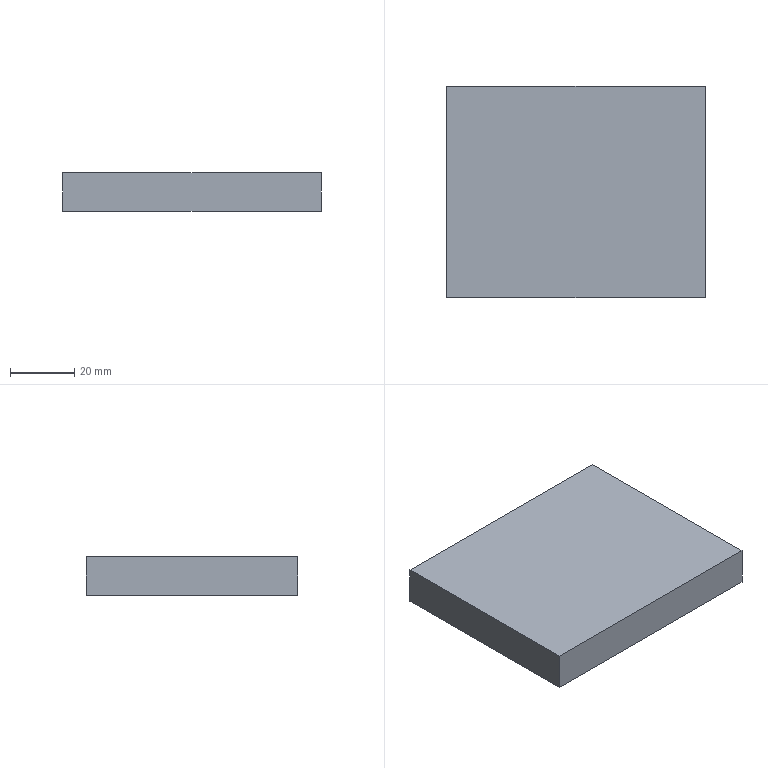Part | SolidWorks | features FlatPattern 1, SMBaseFlange 1, SheetMetal 1 | 1 solid | 6 faces | box 80.7 x 66 x 12 mm | volume 63914 mm3 | plane 6
STEP:
#1=CARTESIAN_POINT('',(-105.455,78.,0.));
#2=VERTEX_POINT('',#1);
#3=CARTESIAN_POINT('',(-105.455,12.,0.));
#4=VERTEX_POINT('',#3);
#5=CARTESIAN_POINT('',(-105.455,12.,0.));
#6=DIRECTION('',(0.,-1.,0.));
#7=VECTOR('',#6,1000.);
#8=LINE('',#5,#7);
#9=EDGE_CURVE('',#2,#4,#8,.T.);
#10=ORIENTED_EDGE('',*,*,#9,.F.);
#11=CARTESIAN_POINT('',(-105.455,78.,-12.));
#12=VERTEX_POINT('',#11);
#13=CARTESIAN_POINT('',(-105.455,78.,-12.));
#14=DIRECTION('',(0.,0.,1.));
#15=VECTOR('',#14,1000.);
#16=LINE('',#13,#15);
#17=EDGE_CURVE('',#12,#2,#16,.T.);
#18=ORIENTED_EDGE('',*,*,#17,.F.);
#19=CARTESIAN_POINT('',(-105.455,12.,-12.));
#20=VERTEX_POINT('',#19);
#21=CARTESIAN_POINT('',(-105.455,12.,-12.));
#22=DIRECTION('',(0.,-1.,0.));
#23=VECTOR('',#22,1000.);
#24=LINE('',#21,#23);
#25=EDGE_CURVE('',#12,#20,#24,.T.);
#26=ORIENTED_EDGE('',*,*,#25,.T.);
#27=CARTESIAN_POINT('',(-105.455,12.,-12.));
#28=DIRECTION('',(0.,0.,1.));
#29=VECTOR('',#28,1000.);
#30=LINE('',#27,#29);
#31=EDGE_CURVE('',#20,#4,#30,.T.);
#32=ORIENTED_EDGE('',*,*,#31,.T.);
#33=EDGE_LOOP('',(#10,#18,#26,#32));
#34=FACE_OUTER_BOUND('',#33,.T.);
#35=CARTESIAN_POINT('',(-105.455,12.,-12.));
#36=DIRECTION('',(-1.,0.,0.));
#37=DIRECTION('',(0.,0.,1.));
#38=AXIS2_PLACEMENT_3D('',#35,#36,#37);
#39=PLANE('',#38);
#40=ADVANCED_FACE('',(#34),#39,.T.);
#41=CARTESIAN_POINT('',(-24.755,78.,0.));
#42=VERTEX_POINT('',#41);
#43=CARTESIAN_POINT('',(-105.455,78.,0.));
#44=DIRECTION('',(-1.,0.,0.));
#45=VECTOR('',#44,1000.);
#46=LINE('',#43,#45);
#47=EDGE_CURVE('',#42,#2,#46,.T.);
#48=ORIENTED_EDGE('',*,*,#47,.F.);
#49=CARTESIAN_POINT('',(-24.755,78.,-12.));
#50=VERTEX_POINT('',#49);
#51=CARTESIAN_POINT('',(-24.755,78.,-12.));
#52=DIRECTION('',(0.,0.,1.));
#53=VECTOR('',#52,1000.);
#54=LINE('',#51,#53);
#55=EDGE_CURVE('',#50,#42,#54,.T.);
#56=ORIENTED_EDGE('',*,*,#55,.F.);
#57=CARTESIAN_POINT('',(-105.455,78.,-12.));
#58=DIRECTION('',(-1.,0.,0.));
#59=VECTOR('',#58,1000.);
#60=LINE('',#57,#59);
#61=EDGE_CURVE('',#50,#12,#60,.T.);
#62=ORIENTED_EDGE('',*,*,#61,.T.);
#63=ORIENTED_EDGE('',*,*,#17,.T.);
#64=EDGE_LOOP('',(#48,#56,#62,#63));
#65=FACE_OUTER_BOUND('',#64,.T.);
#66=CARTESIAN_POINT('',(-105.455,78.,-12.));
#67=DIRECTION('',(0.,1.,0.));
#68=DIRECTION('',(0.,0.,1.));
#69=AXIS2_PLACEMENT_3D('',#66,#67,#68);
#70=PLANE('',#69);
#71=ADVANCED_FACE('',(#65),#70,.T.);
#72=CARTESIAN_POINT('',(-24.755,12.,0.));
#73=VERTEX_POINT('',#72);
#74=CARTESIAN_POINT('',(-24.755,12.,0.));
#75=DIRECTION('',(0.,1.,0.));
#76=VECTOR('',#75,1000.);
#77=LINE('',#74,#76);
#78=EDGE_CURVE('',#73,#42,#77,.T.);
#79=ORIENTED_EDGE('',*,*,#78,.F.);
#80=CARTESIAN_POINT('',(-24.755,12.,-12.));
#81=VERTEX_POINT('',#80);
#82=CARTESIAN_POINT('',(-24.755,12.,-12.));
#83=DIRECTION('',(0.,0.,1.));
#84=VECTOR('',#83,1000.);
#85=LINE('',#82,#84);
#86=EDGE_CURVE('',#81,#73,#85,.T.);
#87=ORIENTED_EDGE('',*,*,#86,.F.);
#88=CARTESIAN_POINT('',(-24.755,12.,-12.));
#89=DIRECTION('',(0.,1.,0.));
#90=VECTOR('',#89,1000.);
#91=LINE('',#88,#90);
#92=EDGE_CURVE('',#81,#50,#91,.T.);
#93=ORIENTED_EDGE('',*,*,#92,.T.);
#94=ORIENTED_EDGE('',*,*,#55,.T.);
#95=EDGE_LOOP('',(#79,#87,#93,#94));
#96=FACE_OUTER_BOUND('',#95,.T.);
#97=CARTESIAN_POINT('',(-24.755,12.,-12.));
#98=DIRECTION('',(1.,0.,0.));
#99=DIRECTION('',(0.,0.,-1.));
#100=AXIS2_PLACEMENT_3D('',#97,#98,#99);
#101=PLANE('',#100);
#102=ADVANCED_FACE('',(#96),#101,.T.);
#103=CARTESIAN_POINT('',(-105.455,12.,0.));
#104=DIRECTION('',(1.,0.,0.));
#105=VECTOR('',#104,1000.);
#106=LINE('',#103,#105);
#107=EDGE_CURVE('',#4,#73,#106,.T.);
#108=ORIENTED_EDGE('',*,*,#107,.F.);
#109=ORIENTED_EDGE('',*,*,#31,.F.);
#110=CARTESIAN_POINT('',(-105.455,12.,-12.));
#111=DIRECTION('',(1.,0.,0.));
#112=VECTOR('',#111,1000.);
#113=LINE('',#110,#112);
#114=EDGE_CURVE('',#20,#81,#113,.T.);
#115=ORIENTED_EDGE('',*,*,#114,.T.);
#116=ORIENTED_EDGE('',*,*,#86,.T.);
#117=EDGE_LOOP('',(#108,#109,#115,#116));
#118=FACE_OUTER_BOUND('',#117,.T.);
#119=CARTESIAN_POINT('',(-105.455,12.,-12.));
#120=DIRECTION('',(0.,-1.,0.));
#121=DIRECTION('',(0.,0.,-1.));
#122=AXIS2_PLACEMENT_3D('',#119,#120,#121);
#123=PLANE('',#122);
#124=ADVANCED_FACE('',(#118),#123,.T.);
#125=ORIENTED_EDGE('',*,*,#25,.F.);
#126=ORIENTED_EDGE('',*,*,#61,.F.);
#127=ORIENTED_EDGE('',*,*,#92,.F.);
#128=ORIENTED_EDGE('',*,*,#114,.F.);
#129=EDGE_LOOP('',(#125,#126,#127,#128));
#130=FACE_OUTER_BOUND('',#129,.T.);
#131=CARTESIAN_POINT('',(0.,0.,-12.));
#132=DIRECTION('',(0.,0.,-1.));
#133=DIRECTION('',(-1.,0.,0.));
#134=AXIS2_PLACEMENT_3D('',#131,#132,#133);
#135=PLANE('',#134);
#136=ADVANCED_FACE('',(#130),#135,.T.);
#137=ORIENTED_EDGE('',*,*,#9,.T.);
#138=ORIENTED_EDGE('',*,*,#107,.T.);
#139=ORIENTED_EDGE('',*,*,#78,.T.);
#140=ORIENTED_EDGE('',*,*,#47,.T.);
#141=EDGE_LOOP('',(#137,#138,#139,#140));
#142=FACE_OUTER_BOUND('',#141,.T.);
#143=CARTESIAN_POINT('',(0.,0.,0.));
#144=DIRECTION('',(0.,0.,-1.));
#145=DIRECTION('',(-1.,0.,0.));
#146=AXIS2_PLACEMENT_3D('',#143,#144,#145);
#147=PLANE('',#146);
#148=ADVANCED_FACE('',(#142),#147,.F.);
#149=CLOSED_SHELL('',(#40,#71,#102,#124,#136,#148));
#150=MANIFOLD_SOLID_BREP('',#149);
#151=CARTESIAN_POINT('',(0.,0.,0.));
#152=DIRECTION('',(0.,0.,1.));
#153=DIRECTION('',(1.,0.,0.));
#154=AXIS2_PLACEMENT_3D('',#151,#152,#153);
#155=(LENGTH_UNIT()NAMED_UNIT(*)SI_UNIT(.MILLI.,.METRE.));
#156=UNCERTAINTY_MEASURE_WITH_UNIT(LENGTH_MEASURE(0.00001),#155,'','');
#157=(NAMED_UNIT(*)PLANE_ANGLE_UNIT()SI_UNIT($,.RADIAN.));
#158=(NAMED_UNIT(*)SI_UNIT($,.STERADIAN.)SOLID_ANGLE_UNIT());
#159=(GEOMETRIC_REPRESENTATION_CONTEXT(3)GLOBAL_UNCERTAINTY_ASSIGNED_CONTEXT((#156))GLOBAL_UNIT_ASSIGNED_CONTEXT((#155,#157,#158))REPRESENTATION_CONTEXT('',''));
#160=ADVANCED_BREP_SHAPE_REPRESENTATION('',(#150,#154),#159);